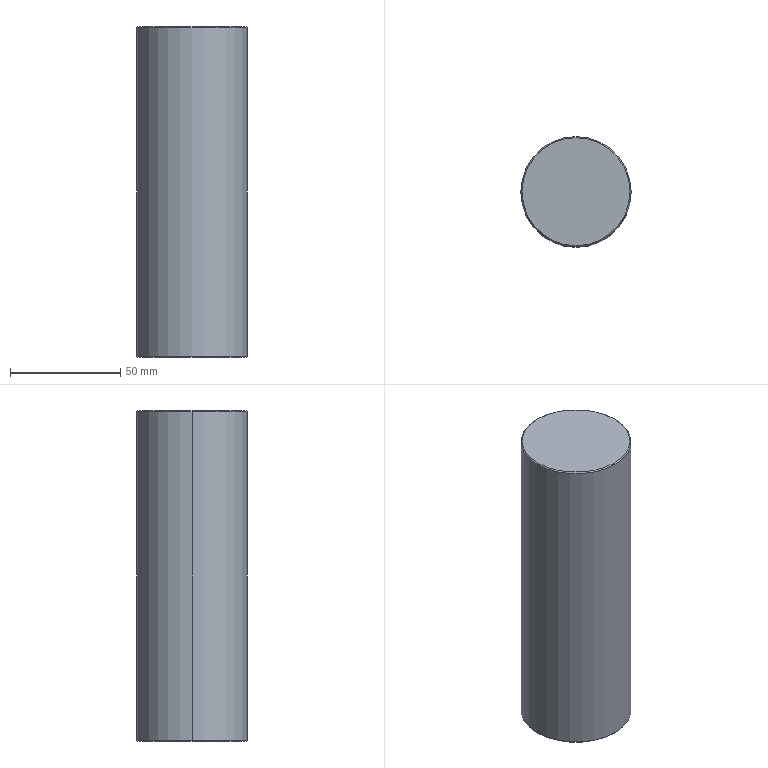Part | Creo | 1 solid | 12 faces | box 50 x 50 x 150 mm | volume 293693 mm3 | cone 6 | cylinder 4 | plane 2 | commonest cylinder face diameters 8 x2 50 x2
STEP:
#1=CARTESIAN_POINT('',(-74.5,-78.,-300.5));
#2=VERTEX_POINT('',#1);
#3=CARTESIAN_POINT('',(-25.5,-78.,-300.5));
#4=VERTEX_POINT('',#3);
#5=CARTESIAN_POINT('',(-50.,-78.,-300.5));
#6=DIRECTION('',(0.,0.,-1.));
#7=DIRECTION('',(-1.,0.,0.));
#8=AXIS2_PLACEMENT_3D('',#5,#6,#7);
#9=CIRCLE('',#8,24.5);
#10=EDGE_CURVE('',#2,#4,#9,.T.);
#11=ORIENTED_EDGE('',*,*,#10,.F.);
#12=CARTESIAN_POINT('',(-50.,-78.,-300.5));
#13=DIRECTION('',(0.,0.,-1.));
#14=DIRECTION('',(1.,0.,0.));
#15=AXIS2_PLACEMENT_3D('',#12,#13,#14);
#16=CIRCLE('',#15,24.5);
#17=EDGE_CURVE('',#4,#2,#16,.T.);
#18=ORIENTED_EDGE('',*,*,#17,.F.);
#19=EDGE_LOOP('',(#11,#18));
#20=FACE_OUTER_BOUND('',#19,.F.);
#21=CARTESIAN_POINT('',(-46.,-78.,-300.5));
#22=VERTEX_POINT('',#21);
#23=CARTESIAN_POINT('',(-54.,-78.,-300.5));
#24=VERTEX_POINT('',#23);
#25=CARTESIAN_POINT('',(-50.,-78.,-300.5));
#26=DIRECTION('',(0.,0.,1.));
#27=DIRECTION('',(1.,0.,0.));
#28=AXIS2_PLACEMENT_3D('',#25,#26,#27);
#29=CIRCLE('',#28,4.);
#30=EDGE_CURVE('',#22,#24,#29,.T.);
#31=ORIENTED_EDGE('',*,*,#30,.F.);
#32=CARTESIAN_POINT('',(-50.,-78.,-300.5));
#33=DIRECTION('',(0.,0.,1.));
#34=DIRECTION('',(-1.,0.,0.));
#35=AXIS2_PLACEMENT_3D('',#32,#33,#34);
#36=CIRCLE('',#35,4.);
#37=EDGE_CURVE('',#24,#22,#36,.T.);
#38=ORIENTED_EDGE('',*,*,#37,.F.);
#39=EDGE_LOOP('',(#31,#38));
#40=FACE_BOUND('',#39,.F.);
#41=CARTESIAN_POINT('',(-50.,-78.,-300.5));
#42=DIRECTION('',(0.,0.,-1.));
#43=DIRECTION('',(-1.,0.,0.));
#44=AXIS2_PLACEMENT_3D('',#41,#42,#43);
#45=PLANE('',#44);
#46=ADVANCED_FACE('',(#20,#40),#45,.T.);
#47=ORIENTED_EDGE('',*,*,#10,.T.);
#48=CARTESIAN_POINT('',(-25.,-78.,-300.));
#49=VERTEX_POINT('',#48);
#50=CARTESIAN_POINT('',(-25.5,-78.,-300.5));
#51=DIRECTION('',(0.7071,0.,0.7071));
#52=VECTOR('',#51,0.7071);
#53=LINE('',#50,#52);
#54=EDGE_CURVE('',#4,#49,#53,.T.);
#55=ORIENTED_EDGE('',*,*,#54,.T.);
#56=CARTESIAN_POINT('',(-75.,-78.,-300.));
#57=VERTEX_POINT('',#56);
#58=CARTESIAN_POINT('',(-50.,-78.,-300.));
#59=DIRECTION('',(0.,0.,-1.));
#60=DIRECTION('',(-1.,0.,0.));
#61=AXIS2_PLACEMENT_3D('',#58,#59,#60);
#62=CIRCLE('',#61,25.);
#63=EDGE_CURVE('',#57,#49,#62,.T.);
#64=ORIENTED_EDGE('',*,*,#63,.F.);
#65=CARTESIAN_POINT('',(-74.5,-78.,-300.5));
#66=DIRECTION('',(-0.7071,0.,0.7071));
#67=VECTOR('',#66,0.7071);
#68=LINE('',#65,#67);
#69=EDGE_CURVE('',#2,#57,#68,.T.);
#70=ORIENTED_EDGE('',*,*,#69,.F.);
#71=EDGE_LOOP('',(#47,#55,#64,#70));
#72=FACE_OUTER_BOUND('',#71,.F.);
#73=CARTESIAN_POINT('',(-50.,-78.,-300.25));
#74=DIRECTION('',(0.,0.,1.));
#75=DIRECTION('',(1.,0.,0.));
#76=AXIS2_PLACEMENT_3D('',#73,#74,#75);
#77=CONICAL_SURFACE('',#76,24.75,45.);
#78=ADVANCED_FACE('',(#72),#77,.T.);
#79=ORIENTED_EDGE('',*,*,#17,.T.);
#80=ORIENTED_EDGE('',*,*,#69,.T.);
#81=CARTESIAN_POINT('',(-50.,-78.,-300.));
#82=DIRECTION('',(0.,0.,-1.));
#83=DIRECTION('',(1.,0.,0.));
#84=AXIS2_PLACEMENT_3D('',#81,#82,#83);
#85=CIRCLE('',#84,25.);
#86=EDGE_CURVE('',#49,#57,#85,.T.);
#87=ORIENTED_EDGE('',*,*,#86,.F.);
#88=ORIENTED_EDGE('',*,*,#54,.F.);
#89=EDGE_LOOP('',(#79,#80,#87,#88));
#90=FACE_OUTER_BOUND('',#89,.F.);
#91=CARTESIAN_POINT('',(-50.,-78.,-300.25));
#92=DIRECTION('',(0.,0.,1.));
#93=DIRECTION('',(1.,0.,0.));
#94=AXIS2_PLACEMENT_3D('',#91,#92,#93);
#95=CONICAL_SURFACE('',#94,24.75,45.);
#96=ADVANCED_FACE('',(#90),#95,.T.);
#97=ORIENTED_EDGE('',*,*,#86,.T.);
#98=CARTESIAN_POINT('',(-75.,-78.,-151.));
#99=VERTEX_POINT('',#98);
#100=CARTESIAN_POINT('',(-75.,-78.,-151.));
#101=DIRECTION('',(0.,0.,-1.));
#102=VECTOR('',#101,149.);
#103=LINE('',#100,#102);
#104=EDGE_CURVE('',#99,#57,#103,.T.);
#105=ORIENTED_EDGE('',*,*,#104,.F.);
#106=CARTESIAN_POINT('',(-25.,-78.,-151.));
#107=VERTEX_POINT('',#106);
#108=CARTESIAN_POINT('',(-50.,-78.,-151.));
#109=DIRECTION('',(0.,0.,1.));
#110=DIRECTION('',(-1.,0.,0.));
#111=AXIS2_PLACEMENT_3D('',#108,#109,#110);
#112=CIRCLE('',#111,25.);
#113=EDGE_CURVE('',#99,#107,#112,.T.);
#114=ORIENTED_EDGE('',*,*,#113,.T.);
#115=CARTESIAN_POINT('',(-25.,-78.,-151.));
#116=DIRECTION('',(0.,0.,-1.));
#117=VECTOR('',#116,149.);
#118=LINE('',#115,#117);
#119=EDGE_CURVE('',#107,#49,#118,.T.);
#120=ORIENTED_EDGE('',*,*,#119,.T.);
#121=EDGE_LOOP('',(#97,#105,#114,#120));
#122=FACE_OUTER_BOUND('',#121,.F.);
#123=CARTESIAN_POINT('',(-50.,-78.,-150.5));
#124=DIRECTION('',(0.,0.,-1.));
#125=DIRECTION('',(-1.,0.,0.));
#126=AXIS2_PLACEMENT_3D('',#123,#124,#125);
#127=CYLINDRICAL_SURFACE('',#126,25.);
#128=ADVANCED_FACE('',(#122),#127,.T.);
#129=ORIENTED_EDGE('',*,*,#63,.T.);
#130=ORIENTED_EDGE('',*,*,#119,.F.);
#131=CARTESIAN_POINT('',(-50.,-78.,-151.));
#132=DIRECTION('',(0.,0.,1.));
#133=DIRECTION('',(1.,0.,0.));
#134=AXIS2_PLACEMENT_3D('',#131,#132,#133);
#135=CIRCLE('',#134,25.);
#136=EDGE_CURVE('',#107,#99,#135,.T.);
#137=ORIENTED_EDGE('',*,*,#136,.T.);
#138=ORIENTED_EDGE('',*,*,#104,.T.);
#139=EDGE_LOOP('',(#129,#130,#137,#138));
#140=FACE_OUTER_BOUND('',#139,.F.);
#141=CARTESIAN_POINT('',(-50.,-78.,-150.5));
#142=DIRECTION('',(0.,0.,-1.));
#143=DIRECTION('',(-1.,0.,0.));
#144=AXIS2_PLACEMENT_3D('',#141,#142,#143);
#145=CYLINDRICAL_SURFACE('',#144,25.);
#146=ADVANCED_FACE('',(#140),#145,.T.);
#147=CARTESIAN_POINT('',(-25.5,-78.,-150.5));
#148=VERTEX_POINT('',#147);
#149=CARTESIAN_POINT('',(-74.5,-78.,-150.5));
#150=VERTEX_POINT('',#149);
#151=CARTESIAN_POINT('',(-50.,-78.,-150.5));
#152=DIRECTION('',(0.,0.,1.));
#153=DIRECTION('',(1.,0.,0.));
#154=AXIS2_PLACEMENT_3D('',#151,#152,#153);
#155=CIRCLE('',#154,24.5);
#156=EDGE_CURVE('',#148,#150,#155,.T.);
#157=ORIENTED_EDGE('',*,*,#156,.T.);
#158=CARTESIAN_POINT('',(-74.5,-78.,-150.5));
#159=DIRECTION('',(-0.7071,0.,-0.7071));
#160=VECTOR('',#159,0.7071);
#161=LINE('',#158,#160);
#162=EDGE_CURVE('',#150,#99,#161,.T.);
#163=ORIENTED_EDGE('',*,*,#162,.T.);
#164=ORIENTED_EDGE('',*,*,#136,.F.);
#165=CARTESIAN_POINT('',(-25.5,-78.,-150.5));
#166=DIRECTION('',(0.7071,0.,-0.7071));
#167=VECTOR('',#166,0.7071);
#168=LINE('',#165,#167);
#169=EDGE_CURVE('',#148,#107,#168,.T.);
#170=ORIENTED_EDGE('',*,*,#169,.F.);
#171=EDGE_LOOP('',(#157,#163,#164,#170));
#172=FACE_OUTER_BOUND('',#171,.F.);
#173=CARTESIAN_POINT('',(-50.,-78.,-150.75));
#174=DIRECTION('',(0.,0.,-1.));
#175=DIRECTION('',(-1.,0.,0.));
#176=AXIS2_PLACEMENT_3D('',#173,#174,#175);
#177=CONICAL_SURFACE('',#176,24.75,45.);
#178=ADVANCED_FACE('',(#172),#177,.T.);
#179=ORIENTED_EDGE('',*,*,#156,.F.);
#180=CARTESIAN_POINT('',(-50.,-78.,-150.5));
#181=DIRECTION('',(0.,0.,1.));
#182=DIRECTION('',(-1.,0.,0.));
#183=AXIS2_PLACEMENT_3D('',#180,#181,#182);
#184=CIRCLE('',#183,24.5);
#185=EDGE_CURVE('',#150,#148,#184,.T.);
#186=ORIENTED_EDGE('',*,*,#185,.F.);
#187=EDGE_LOOP('',(#179,#186));
#188=FACE_OUTER_BOUND('',#187,.F.);
#189=CARTESIAN_POINT('',(-50.,-78.,-150.5));
#190=DIRECTION('',(0.,0.,1.));
#191=DIRECTION('',(1.,0.,0.));
#192=AXIS2_PLACEMENT_3D('',#189,#190,#191);
#193=PLANE('',#192);
#194=ADVANCED_FACE('',(#188),#193,.T.);
#195=ORIENTED_EDGE('',*,*,#185,.T.);
#196=ORIENTED_EDGE('',*,*,#169,.T.);
#197=ORIENTED_EDGE('',*,*,#113,.F.);
#198=ORIENTED_EDGE('',*,*,#162,.F.);
#199=EDGE_LOOP('',(#195,#196,#197,#198));
#200=FACE_OUTER_BOUND('',#199,.F.);
#201=CARTESIAN_POINT('',(-50.,-78.,-150.75));
#202=DIRECTION('',(0.,0.,-1.));
#203=DIRECTION('',(-1.,0.,0.));
#204=AXIS2_PLACEMENT_3D('',#201,#202,#203);
#205=CONICAL_SURFACE('',#204,24.75,45.);
#206=ADVANCED_FACE('',(#200),#205,.T.);
#207=CARTESIAN_POINT('',(-54.,-78.,-285.5));
#208=VERTEX_POINT('',#207);
#209=CARTESIAN_POINT('',(-46.,-78.,-285.5));
#210=VERTEX_POINT('',#209);
#211=CARTESIAN_POINT('',(-50.,-78.,-285.5));
#212=DIRECTION('',(0.,0.,-1.));
#213=DIRECTION('',(-1.,0.,0.));
#214=AXIS2_PLACEMENT_3D('',#211,#212,#213);
#215=CIRCLE('',#214,4.);
#216=EDGE_CURVE('',#208,#210,#215,.T.);
#217=ORIENTED_EDGE('',*,*,#216,.T.);
#218=CARTESIAN_POINT('',(-46.,-78.,-300.5));
#219=DIRECTION('',(0.,0.,1.));
#220=VECTOR('',#219,15.);
#221=LINE('',#218,#220);
#222=EDGE_CURVE('',#22,#210,#221,.T.);
#223=ORIENTED_EDGE('',*,*,#222,.F.);
#224=ORIENTED_EDGE('',*,*,#30,.T.);
#225=CARTESIAN_POINT('',(-54.,-78.,-300.5));
#226=DIRECTION('',(0.,0.,1.));
#227=VECTOR('',#226,15.);
#228=LINE('',#225,#227);
#229=EDGE_CURVE('',#24,#208,#228,.T.);
#230=ORIENTED_EDGE('',*,*,#229,.T.);
#231=EDGE_LOOP('',(#217,#223,#224,#230));
#232=FACE_OUTER_BOUND('',#231,.F.);
#233=CARTESIAN_POINT('',(-50.,-78.,-300.5));
#234=DIRECTION('',(0.,0.,1.));
#235=DIRECTION('',(1.,0.,0.));
#236=AXIS2_PLACEMENT_3D('',#233,#234,#235);
#237=CYLINDRICAL_SURFACE('',#236,4.);
#238=ADVANCED_FACE('',(#232),#237,.F.);
#239=ORIENTED_EDGE('',*,*,#216,.F.);
#240=CARTESIAN_POINT('',(-50.,-78.,-283.19));
#241=VERTEX_POINT('',#240);
#242=CARTESIAN_POINT('',(-50.,-78.,-283.19));
#243=DIRECTION('',(-0.866,0.,-0.5001));
#244=VECTOR('',#243,4.619);
#245=LINE('',#242,#244);
#246=EDGE_CURVE('',#241,#208,#245,.T.);
#247=ORIENTED_EDGE('',*,*,#246,.F.);
#248=CARTESIAN_POINT('',(-50.,-78.,-283.19));
#249=DIRECTION('',(0.866,0.,-0.5001));
#250=VECTOR('',#249,4.619);
#251=LINE('',#248,#250);
#252=EDGE_CURVE('',#241,#210,#251,.T.);
#253=ORIENTED_EDGE('',*,*,#252,.T.);
#254=EDGE_LOOP('',(#239,#247,#253));
#255=FACE_OUTER_BOUND('',#254,.F.);
#256=CARTESIAN_POINT('',(-50.,-78.,-284.395));
#257=DIRECTION('',(0.,0.,-1.));
#258=DIRECTION('',(-1.,0.,0.));
#259=AXIS2_PLACEMENT_3D('',#256,#257,#258);
#260=CONICAL_SURFACE('',#259,2.086,59.994);
#261=ADVANCED_FACE('',(#255),#260,.F.);
#262=CARTESIAN_POINT('',(-50.,-78.,-285.5));
#263=DIRECTION('',(0.,0.,-1.));
#264=DIRECTION('',(1.,0.,0.));
#265=AXIS2_PLACEMENT_3D('',#262,#263,#264);
#266=CIRCLE('',#265,4.);
#267=EDGE_CURVE('',#210,#208,#266,.T.);
#268=ORIENTED_EDGE('',*,*,#267,.F.);
#269=ORIENTED_EDGE('',*,*,#252,.F.);
#270=ORIENTED_EDGE('',*,*,#246,.T.);
#271=EDGE_LOOP('',(#268,#269,#270));
#272=FACE_OUTER_BOUND('',#271,.F.);
#273=CARTESIAN_POINT('',(-50.,-78.,-284.395));
#274=DIRECTION('',(0.,0.,-1.));
#275=DIRECTION('',(-1.,0.,0.));
#276=AXIS2_PLACEMENT_3D('',#273,#274,#275);
#277=CONICAL_SURFACE('',#276,2.086,59.994);
#278=ADVANCED_FACE('',(#272),#277,.F.);
#279=ORIENTED_EDGE('',*,*,#267,.T.);
#280=ORIENTED_EDGE('',*,*,#229,.F.);
#281=ORIENTED_EDGE('',*,*,#37,.T.);
#282=ORIENTED_EDGE('',*,*,#222,.T.);
#283=EDGE_LOOP('',(#279,#280,#281,#282));
#284=FACE_OUTER_BOUND('',#283,.F.);
#285=CARTESIAN_POINT('',(-50.,-78.,-300.5));
#286=DIRECTION('',(0.,0.,1.));
#287=DIRECTION('',(1.,0.,0.));
#288=AXIS2_PLACEMENT_3D('',#285,#286,#287);
#289=CYLINDRICAL_SURFACE('',#288,4.);
#290=ADVANCED_FACE('',(#284),#289,.F.);
#291=CLOSED_SHELL('',(#46,#78,#96,#128,#146,#178,#194,#206,#238,#261,#278,#290));
#292=MANIFOLD_SOLID_BREP('',#291);
#293=(LENGTH_UNIT()NAMED_UNIT(*)SI_UNIT(.MILLI.,.METRE.));
#294=UNCERTAINTY_MEASURE_WITH_UNIT(LENGTH_MEASURE(0.01658),#293,'','');
#295=(NAMED_UNIT(*)PLANE_ANGLE_UNIT()SI_UNIT($,.RADIAN.));
#296=PLANE_ANGLE_MEASURE_WITH_UNIT(PLANE_ANGLE_MEASURE(0.01745),#295);
#297=(CONVERSION_BASED_UNIT('DEGREE',#296)NAMED_UNIT(*)PLANE_ANGLE_UNIT());
#298=(NAMED_UNIT(*)SI_UNIT($,.STERADIAN.)SOLID_ANGLE_UNIT());
#299=(GEOMETRIC_REPRESENTATION_CONTEXT(3)GLOBAL_UNCERTAINTY_ASSIGNED_CONTEXT((#294))GLOBAL_UNIT_ASSIGNED_CONTEXT((#293,#297,#298))REPRESENTATION_CONTEXT('',''));
#300=ADVANCED_BREP_SHAPE_REPRESENTATION('',(#292),#299);